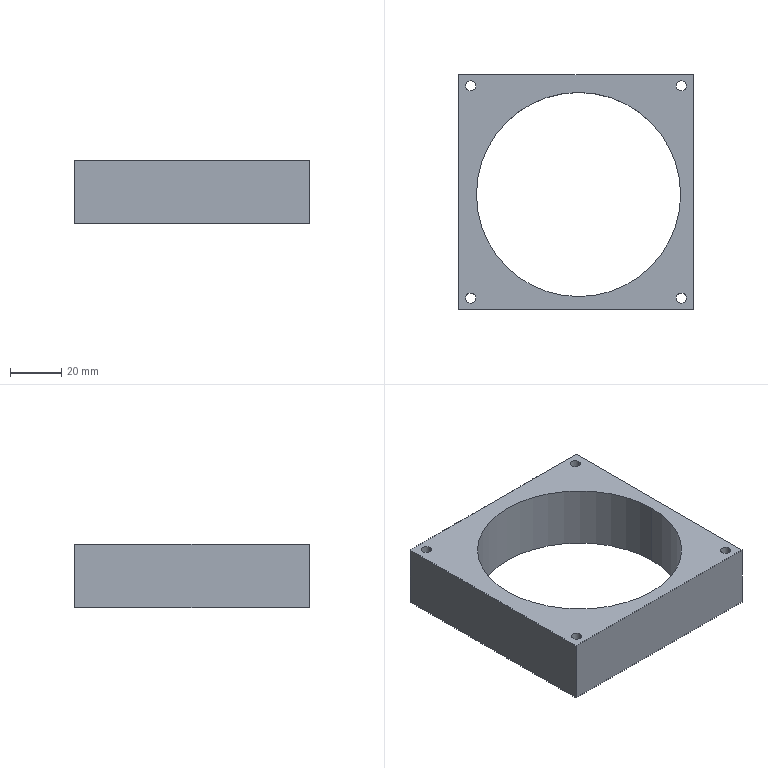Part | SolidWorks | features ICE 2, Extrusion 1 | 1 solid | 16 faces | box 92 x 92 x 25 mm | volume 84680 mm3 | cylinder 10 | plane 6 | commonest cylinder face diameters 4 x8 80 x2
STEP:
#1=CARTESIAN_POINT('',(-6.75,4.4,0.));
#2=VERTEX_POINT('',#1);
#3=CARTESIAN_POINT('',(-2.75,4.4,0.));
#4=VERTEX_POINT('',#3);
#5=CARTESIAN_POINT('',(-4.75,4.4,0.));
#6=DIRECTION('',(0.,0.,1.));
#7=DIRECTION('',(1.,0.,0.));
#8=AXIS2_PLACEMENT_3D('',#5,#6,#7);
#9=CIRCLE('',#8,2.);
#10=EDGE_CURVE('',#2,#4,#9,.T.);
#11=ORIENTED_EDGE('',*,*,#10,.F.);
#12=CARTESIAN_POINT('',(-6.75,4.4,25.));
#13=VERTEX_POINT('',#12);
#14=CARTESIAN_POINT('',(-6.75,4.4,-5.));
#15=DIRECTION('',(0.,0.,1.));
#16=VECTOR('',#15,1000.);
#17=LINE('',#14,#16);
#18=EDGE_CURVE('',#2,#13,#17,.T.);
#19=ORIENTED_EDGE('',*,*,#18,.T.);
#20=CARTESIAN_POINT('',(-2.75,4.4,25.));
#21=VERTEX_POINT('',#20);
#22=CARTESIAN_POINT('',(-4.75,4.4,25.));
#23=DIRECTION('',(0.,0.,1.));
#24=DIRECTION('',(-1.,0.,0.));
#25=AXIS2_PLACEMENT_3D('',#22,#23,#24);
#26=CIRCLE('',#25,2.);
#27=EDGE_CURVE('',#13,#21,#26,.T.);
#28=ORIENTED_EDGE('',*,*,#27,.T.);
#29=CARTESIAN_POINT('',(-2.75,4.4,-5.));
#30=DIRECTION('',(0.,0.,1.));
#31=VECTOR('',#30,1000.);
#32=LINE('',#29,#31);
#33=EDGE_CURVE('',#4,#21,#32,.T.);
#34=ORIENTED_EDGE('',*,*,#33,.F.);
#35=EDGE_LOOP('',(#11,#19,#28,#34));
#36=FACE_OUTER_BOUND('',#35,.T.);
#37=CARTESIAN_POINT('',(-4.75,4.4,-5.));
#38=DIRECTION('',(0.,0.,1.));
#39=DIRECTION('',(1.,0.,0.));
#40=AXIS2_PLACEMENT_3D('',#37,#38,#39);
#41=CYLINDRICAL_SURFACE('',#40,2.);
#42=ADVANCED_FACE('',(#36),#41,.F.);
#43=CARTESIAN_POINT('',(-89.25,4.4,0.));
#44=VERTEX_POINT('',#43);
#45=CARTESIAN_POINT('',(-85.25,4.4,0.));
#46=VERTEX_POINT('',#45);
#47=CARTESIAN_POINT('',(-87.25,4.4,0.));
#48=DIRECTION('',(0.,0.,1.));
#49=DIRECTION('',(1.,0.,0.));
#50=AXIS2_PLACEMENT_3D('',#47,#48,#49);
#51=CIRCLE('',#50,2.);
#52=EDGE_CURVE('',#44,#46,#51,.T.);
#53=ORIENTED_EDGE('',*,*,#52,.F.);
#54=CARTESIAN_POINT('',(-89.25,4.4,25.));
#55=VERTEX_POINT('',#54);
#56=CARTESIAN_POINT('',(-89.25,4.4,-5.));
#57=DIRECTION('',(0.,0.,1.));
#58=VECTOR('',#57,1000.);
#59=LINE('',#56,#58);
#60=EDGE_CURVE('',#44,#55,#59,.T.);
#61=ORIENTED_EDGE('',*,*,#60,.T.);
#62=CARTESIAN_POINT('',(-85.25,4.4,25.));
#63=VERTEX_POINT('',#62);
#64=CARTESIAN_POINT('',(-87.25,4.4,25.));
#65=DIRECTION('',(0.,0.,1.));
#66=DIRECTION('',(-1.,0.,0.));
#67=AXIS2_PLACEMENT_3D('',#64,#65,#66);
#68=CIRCLE('',#67,2.);
#69=EDGE_CURVE('',#55,#63,#68,.T.);
#70=ORIENTED_EDGE('',*,*,#69,.T.);
#71=CARTESIAN_POINT('',(-85.25,4.4,-5.));
#72=DIRECTION('',(0.,0.,1.));
#73=VECTOR('',#72,1000.);
#74=LINE('',#71,#73);
#75=EDGE_CURVE('',#46,#63,#74,.T.);
#76=ORIENTED_EDGE('',*,*,#75,.F.);
#77=EDGE_LOOP('',(#53,#61,#70,#76));
#78=FACE_OUTER_BOUND('',#77,.T.);
#79=CARTESIAN_POINT('',(-87.25,4.4,-5.));
#80=DIRECTION('',(0.,0.,1.));
#81=DIRECTION('',(1.,0.,0.));
#82=AXIS2_PLACEMENT_3D('',#79,#80,#81);
#83=CYLINDRICAL_SURFACE('',#82,2.);
#84=ADVANCED_FACE('',(#78),#83,.F.);
#85=CARTESIAN_POINT('',(-89.25,87.6,0.));
#86=VERTEX_POINT('',#85);
#87=CARTESIAN_POINT('',(-85.25,87.6,0.));
#88=VERTEX_POINT('',#87);
#89=CARTESIAN_POINT('',(-87.25,87.6,0.));
#90=DIRECTION('',(0.,0.,1.));
#91=DIRECTION('',(1.,0.,0.));
#92=AXIS2_PLACEMENT_3D('',#89,#90,#91);
#93=CIRCLE('',#92,2.);
#94=EDGE_CURVE('',#86,#88,#93,.T.);
#95=ORIENTED_EDGE('',*,*,#94,.F.);
#96=CARTESIAN_POINT('',(-89.25,87.6,25.));
#97=VERTEX_POINT('',#96);
#98=CARTESIAN_POINT('',(-89.25,87.6,-5.));
#99=DIRECTION('',(0.,0.,1.));
#100=VECTOR('',#99,1000.);
#101=LINE('',#98,#100);
#102=EDGE_CURVE('',#86,#97,#101,.T.);
#103=ORIENTED_EDGE('',*,*,#102,.T.);
#104=CARTESIAN_POINT('',(-85.25,87.6,25.));
#105=VERTEX_POINT('',#104);
#106=CARTESIAN_POINT('',(-87.25,87.6,25.));
#107=DIRECTION('',(0.,0.,1.));
#108=DIRECTION('',(1.,0.,0.));
#109=AXIS2_PLACEMENT_3D('',#106,#107,#108);
#110=CIRCLE('',#109,2.);
#111=EDGE_CURVE('',#97,#105,#110,.T.);
#112=ORIENTED_EDGE('',*,*,#111,.T.);
#113=CARTESIAN_POINT('',(-85.25,87.6,-5.));
#114=DIRECTION('',(0.,0.,1.));
#115=VECTOR('',#114,1000.);
#116=LINE('',#113,#115);
#117=EDGE_CURVE('',#88,#105,#116,.T.);
#118=ORIENTED_EDGE('',*,*,#117,.F.);
#119=EDGE_LOOP('',(#95,#103,#112,#118));
#120=FACE_OUTER_BOUND('',#119,.T.);
#121=CARTESIAN_POINT('',(-87.25,87.6,-5.));
#122=DIRECTION('',(0.,0.,1.));
#123=DIRECTION('',(1.,0.,0.));
#124=AXIS2_PLACEMENT_3D('',#121,#122,#123);
#125=CYLINDRICAL_SURFACE('',#124,2.);
#126=ADVANCED_FACE('',(#120),#125,.F.);
#127=CARTESIAN_POINT('',(-6.75,87.6,0.));
#128=VERTEX_POINT('',#127);
#129=CARTESIAN_POINT('',(-2.75,87.6,0.));
#130=VERTEX_POINT('',#129);
#131=CARTESIAN_POINT('',(-4.75,87.6,0.));
#132=DIRECTION('',(0.,0.,1.));
#133=DIRECTION('',(1.,0.,0.));
#134=AXIS2_PLACEMENT_3D('',#131,#132,#133);
#135=CIRCLE('',#134,2.);
#136=EDGE_CURVE('',#128,#130,#135,.T.);
#137=ORIENTED_EDGE('',*,*,#136,.F.);
#138=CARTESIAN_POINT('',(-6.75,87.6,25.));
#139=VERTEX_POINT('',#138);
#140=CARTESIAN_POINT('',(-6.75,87.6,-5.));
#141=DIRECTION('',(0.,0.,1.));
#142=VECTOR('',#141,1000.);
#143=LINE('',#140,#142);
#144=EDGE_CURVE('',#128,#139,#143,.T.);
#145=ORIENTED_EDGE('',*,*,#144,.T.);
#146=CARTESIAN_POINT('',(-2.75,87.6,25.));
#147=VERTEX_POINT('',#146);
#148=CARTESIAN_POINT('',(-4.75,87.6,25.));
#149=DIRECTION('',(0.,0.,1.));
#150=DIRECTION('',(1.,0.,0.));
#151=AXIS2_PLACEMENT_3D('',#148,#149,#150);
#152=CIRCLE('',#151,2.);
#153=EDGE_CURVE('',#139,#147,#152,.T.);
#154=ORIENTED_EDGE('',*,*,#153,.T.);
#155=CARTESIAN_POINT('',(-2.75,87.6,-5.));
#156=DIRECTION('',(0.,0.,1.));
#157=VECTOR('',#156,1000.);
#158=LINE('',#155,#157);
#159=EDGE_CURVE('',#130,#147,#158,.T.);
#160=ORIENTED_EDGE('',*,*,#159,.F.);
#161=EDGE_LOOP('',(#137,#145,#154,#160));
#162=FACE_OUTER_BOUND('',#161,.T.);
#163=CARTESIAN_POINT('',(-4.75,87.6,-5.));
#164=DIRECTION('',(0.,0.,1.));
#165=DIRECTION('',(1.,0.,0.));
#166=AXIS2_PLACEMENT_3D('',#163,#164,#165);
#167=CYLINDRICAL_SURFACE('',#166,2.);
#168=ADVANCED_FACE('',(#162),#167,.F.);
#169=CARTESIAN_POINT('',(-85.,45.,0.));
#170=VERTEX_POINT('',#169);
#171=CARTESIAN_POINT('',(-5.,45.,0.));
#172=VERTEX_POINT('',#171);
#173=CARTESIAN_POINT('',(-45.,45.,0.));
#174=DIRECTION('',(0.,0.,1.));
#175=DIRECTION('',(1.,0.,0.));
#176=AXIS2_PLACEMENT_3D('',#173,#174,#175);
#177=CIRCLE('',#176,40.);
#178=EDGE_CURVE('',#170,#172,#177,.T.);
#179=ORIENTED_EDGE('',*,*,#178,.F.);
#180=CARTESIAN_POINT('',(-85.,45.,25.));
#181=VERTEX_POINT('',#180);
#182=CARTESIAN_POINT('',(-85.,45.,0.));
#183=DIRECTION('',(0.,0.,1.));
#184=VECTOR('',#183,1000.);
#185=LINE('',#182,#184);
#186=EDGE_CURVE('',#170,#181,#185,.T.);
#187=ORIENTED_EDGE('',*,*,#186,.T.);
#188=CARTESIAN_POINT('',(-5.,45.,25.));
#189=VERTEX_POINT('',#188);
#190=CARTESIAN_POINT('',(-45.,45.,25.));
#191=DIRECTION('',(0.,0.,1.));
#192=DIRECTION('',(1.,0.,0.));
#193=AXIS2_PLACEMENT_3D('',#190,#191,#192);
#194=CIRCLE('',#193,40.);
#195=EDGE_CURVE('',#181,#189,#194,.T.);
#196=ORIENTED_EDGE('',*,*,#195,.T.);
#197=CARTESIAN_POINT('',(-5.,45.,0.));
#198=DIRECTION('',(0.,0.,1.));
#199=VECTOR('',#198,1000.);
#200=LINE('',#197,#199);
#201=EDGE_CURVE('',#172,#189,#200,.T.);
#202=ORIENTED_EDGE('',*,*,#201,.F.);
#203=EDGE_LOOP('',(#179,#187,#196,#202));
#204=FACE_OUTER_BOUND('',#203,.T.);
#205=CARTESIAN_POINT('',(-45.,45.,0.));
#206=DIRECTION('',(0.,0.,1.));
#207=DIRECTION('',(1.,0.,0.));
#208=AXIS2_PLACEMENT_3D('',#205,#206,#207);
#209=CYLINDRICAL_SURFACE('',#208,40.);
#210=ADVANCED_FACE('',(#204),#209,.F.);
#211=CARTESIAN_POINT('',(0.,0.,0.));
#212=VERTEX_POINT('',#211);
#213=CARTESIAN_POINT('',(0.,92.,0.));
#214=VERTEX_POINT('',#213);
#215=CARTESIAN_POINT('',(0.,0.,0.));
#216=DIRECTION('',(0.,1.,0.));
#217=VECTOR('',#216,1000.);
#218=LINE('',#215,#217);
#219=EDGE_CURVE('',#212,#214,#218,.T.);
#220=ORIENTED_EDGE('',*,*,#219,.T.);
#221=CARTESIAN_POINT('',(0.,92.,25.));
#222=VERTEX_POINT('',#221);
#223=CARTESIAN_POINT('',(0.,92.,25.));
#224=DIRECTION('',(0.,0.,-1.));
#225=VECTOR('',#224,1000.);
#226=LINE('',#223,#225);
#227=EDGE_CURVE('',#222,#214,#226,.T.);
#228=ORIENTED_EDGE('',*,*,#227,.F.);
#229=CARTESIAN_POINT('',(0.,0.,25.));
#230=VERTEX_POINT('',#229);
#231=CARTESIAN_POINT('',(0.,0.,25.));
#232=DIRECTION('',(0.,1.,0.));
#233=VECTOR('',#232,1000.);
#234=LINE('',#231,#233);
#235=EDGE_CURVE('',#230,#222,#234,.T.);
#236=ORIENTED_EDGE('',*,*,#235,.F.);
#237=CARTESIAN_POINT('',(0.,0.,25.));
#238=DIRECTION('',(0.,0.,-1.));
#239=VECTOR('',#238,1000.);
#240=LINE('',#237,#239);
#241=EDGE_CURVE('',#230,#212,#240,.T.);
#242=ORIENTED_EDGE('',*,*,#241,.T.);
#243=EDGE_LOOP('',(#220,#228,#236,#242));
#244=FACE_OUTER_BOUND('',#243,.T.);
#245=CARTESIAN_POINT('',(0.,0.,25.));
#246=DIRECTION('',(-1.,0.,0.));
#247=DIRECTION('',(0.,-1.,0.));
#248=AXIS2_PLACEMENT_3D('',#245,#246,#247);
#249=PLANE('',#248);
#250=ADVANCED_FACE('',(#244),#249,.F.);
#251=CARTESIAN_POINT('',(-92.,92.,0.));
#252=VERTEX_POINT('',#251);
#253=CARTESIAN_POINT('',(0.,92.,0.));
#254=DIRECTION('',(-1.,0.,0.));
#255=VECTOR('',#254,1000.);
#256=LINE('',#253,#255);
#257=EDGE_CURVE('',#214,#252,#256,.T.);
#258=ORIENTED_EDGE('',*,*,#257,.T.);
#259=CARTESIAN_POINT('',(-92.,92.,25.));
#260=VERTEX_POINT('',#259);
#261=CARTESIAN_POINT('',(-92.,92.,25.));
#262=DIRECTION('',(0.,0.,-1.));
#263=VECTOR('',#262,1000.);
#264=LINE('',#261,#263);
#265=EDGE_CURVE('',#260,#252,#264,.T.);
#266=ORIENTED_EDGE('',*,*,#265,.F.);
#267=CARTESIAN_POINT('',(0.,92.,25.));
#268=DIRECTION('',(-1.,0.,0.));
#269=VECTOR('',#268,1000.);
#270=LINE('',#267,#269);
#271=EDGE_CURVE('',#222,#260,#270,.T.);
#272=ORIENTED_EDGE('',*,*,#271,.F.);
#273=ORIENTED_EDGE('',*,*,#227,.T.);
#274=EDGE_LOOP('',(#258,#266,#272,#273));
#275=FACE_OUTER_BOUND('',#274,.T.);
#276=CARTESIAN_POINT('',(0.,92.,25.));
#277=DIRECTION('',(0.,-1.,0.));
#278=DIRECTION('',(0.,0.,-1.));
#279=AXIS2_PLACEMENT_3D('',#276,#277,#278);
#280=PLANE('',#279);
#281=ADVANCED_FACE('',(#275),#280,.F.);
#282=CARTESIAN_POINT('',(-92.,0.,0.));
#283=VERTEX_POINT('',#282);
#284=CARTESIAN_POINT('',(-92.,0.,0.));
#285=DIRECTION('',(0.,-1.,0.));
#286=VECTOR('',#285,1000.);
#287=LINE('',#284,#286);
#288=EDGE_CURVE('',#252,#283,#287,.T.);
#289=ORIENTED_EDGE('',*,*,#288,.T.);
#290=CARTESIAN_POINT('',(-92.,0.,25.));
#291=VERTEX_POINT('',#290);
#292=CARTESIAN_POINT('',(-92.,0.,25.));
#293=DIRECTION('',(0.,0.,-1.));
#294=VECTOR('',#293,1000.);
#295=LINE('',#292,#294);
#296=EDGE_CURVE('',#291,#283,#295,.T.);
#297=ORIENTED_EDGE('',*,*,#296,.F.);
#298=CARTESIAN_POINT('',(-92.,0.,25.));
#299=DIRECTION('',(0.,-1.,0.));
#300=VECTOR('',#299,1000.);
#301=LINE('',#298,#300);
#302=EDGE_CURVE('',#260,#291,#301,.T.);
#303=ORIENTED_EDGE('',*,*,#302,.F.);
#304=ORIENTED_EDGE('',*,*,#265,.T.);
#305=EDGE_LOOP('',(#289,#297,#303,#304));
#306=FACE_OUTER_BOUND('',#305,.T.);
#307=CARTESIAN_POINT('',(-92.,0.,25.));
#308=DIRECTION('',(1.,0.,0.));
#309=DIRECTION('',(0.,1.,0.));
#310=AXIS2_PLACEMENT_3D('',#307,#308,#309);
#311=PLANE('',#310);
#312=ADVANCED_FACE('',(#306),#311,.F.);
#313=CARTESIAN_POINT('',(0.,0.,0.));
#314=DIRECTION('',(1.,0.,0.));
#315=VECTOR('',#314,1000.);
#316=LINE('',#313,#315);
#317=EDGE_CURVE('',#283,#212,#316,.T.);
#318=ORIENTED_EDGE('',*,*,#317,.T.);
#319=ORIENTED_EDGE('',*,*,#241,.F.);
#320=CARTESIAN_POINT('',(0.,0.,25.));
#321=DIRECTION('',(1.,0.,0.));
#322=VECTOR('',#321,1000.);
#323=LINE('',#320,#322);
#324=EDGE_CURVE('',#291,#230,#323,.T.);
#325=ORIENTED_EDGE('',*,*,#324,.F.);
#326=ORIENTED_EDGE('',*,*,#296,.T.);
#327=EDGE_LOOP('',(#318,#319,#325,#326));
#328=FACE_OUTER_BOUND('',#327,.T.);
#329=CARTESIAN_POINT('',(0.,0.,25.));
#330=DIRECTION('',(0.,1.,0.));
#331=DIRECTION('',(-1.,0.,0.));
#332=AXIS2_PLACEMENT_3D('',#329,#330,#331);
#333=PLANE('',#332);
#334=ADVANCED_FACE('',(#328),#333,.F.);
#335=CARTESIAN_POINT('',(-4.75,4.4,25.));
#336=DIRECTION('',(0.,0.,1.));
#337=DIRECTION('',(-1.,0.,0.));
#338=AXIS2_PLACEMENT_3D('',#335,#336,#337);
#339=CIRCLE('',#338,2.);
#340=EDGE_CURVE('',#21,#13,#339,.T.);
#341=ORIENTED_EDGE('',*,*,#340,.F.);
#342=ORIENTED_EDGE('',*,*,#27,.F.);
#343=EDGE_LOOP('',(#341,#342));
#344=FACE_BOUND('',#343,.T.);
#345=CARTESIAN_POINT('',(-87.25,4.4,25.));
#346=DIRECTION('',(0.,0.,1.));
#347=DIRECTION('',(-1.,0.,0.));
#348=AXIS2_PLACEMENT_3D('',#345,#346,#347);
#349=CIRCLE('',#348,2.);
#350=EDGE_CURVE('',#63,#55,#349,.T.);
#351=ORIENTED_EDGE('',*,*,#350,.F.);
#352=ORIENTED_EDGE('',*,*,#69,.F.);
#353=EDGE_LOOP('',(#351,#352));
#354=FACE_BOUND('',#353,.T.);
#355=CARTESIAN_POINT('',(-87.25,87.6,25.));
#356=DIRECTION('',(0.,0.,1.));
#357=DIRECTION('',(1.,0.,0.));
#358=AXIS2_PLACEMENT_3D('',#355,#356,#357);
#359=CIRCLE('',#358,2.);
#360=EDGE_CURVE('',#105,#97,#359,.T.);
#361=ORIENTED_EDGE('',*,*,#360,.F.);
#362=ORIENTED_EDGE('',*,*,#111,.F.);
#363=EDGE_LOOP('',(#361,#362));
#364=FACE_BOUND('',#363,.T.);
#365=CARTESIAN_POINT('',(-4.75,87.6,25.));
#366=DIRECTION('',(0.,0.,1.));
#367=DIRECTION('',(1.,0.,0.));
#368=AXIS2_PLACEMENT_3D('',#365,#366,#367);
#369=CIRCLE('',#368,2.);
#370=EDGE_CURVE('',#147,#139,#369,.T.);
#371=ORIENTED_EDGE('',*,*,#370,.F.);
#372=ORIENTED_EDGE('',*,*,#153,.F.);
#373=EDGE_LOOP('',(#371,#372));
#374=FACE_BOUND('',#373,.T.);
#375=CARTESIAN_POINT('',(-45.,45.,25.));
#376=DIRECTION('',(0.,0.,1.));
#377=DIRECTION('',(1.,0.,0.));
#378=AXIS2_PLACEMENT_3D('',#375,#376,#377);
#379=CIRCLE('',#378,40.);
#380=EDGE_CURVE('',#189,#181,#379,.T.);
#381=ORIENTED_EDGE('',*,*,#380,.F.);
#382=ORIENTED_EDGE('',*,*,#195,.F.);
#383=EDGE_LOOP('',(#381,#382));
#384=FACE_BOUND('',#383,.T.);
#385=ORIENTED_EDGE('',*,*,#235,.T.);
#386=ORIENTED_EDGE('',*,*,#271,.T.);
#387=ORIENTED_EDGE('',*,*,#302,.T.);
#388=ORIENTED_EDGE('',*,*,#324,.T.);
#389=EDGE_LOOP('',(#385,#386,#387,#388));
#390=FACE_OUTER_BOUND('',#389,.T.);
#391=CARTESIAN_POINT('',(0.,0.,25.));
#392=DIRECTION('',(0.,0.,1.));
#393=DIRECTION('',(1.,0.,0.));
#394=AXIS2_PLACEMENT_3D('',#391,#392,#393);
#395=PLANE('',#394);
#396=ADVANCED_FACE('',(#344,#354,#364,#374,#384,#390),#395,.T.);
#397=CARTESIAN_POINT('',(-4.75,4.4,0.));
#398=DIRECTION('',(0.,0.,1.));
#399=DIRECTION('',(1.,0.,0.));
#400=AXIS2_PLACEMENT_3D('',#397,#398,#399);
#401=CIRCLE('',#400,2.);
#402=EDGE_CURVE('',#4,#2,#401,.T.);
#403=ORIENTED_EDGE('',*,*,#402,.T.);
#404=ORIENTED_EDGE('',*,*,#10,.T.);
#405=EDGE_LOOP('',(#403,#404));
#406=FACE_BOUND('',#405,.T.);
#407=CARTESIAN_POINT('',(-87.25,4.4,0.));
#408=DIRECTION('',(0.,0.,1.));
#409=DIRECTION('',(1.,0.,0.));
#410=AXIS2_PLACEMENT_3D('',#407,#408,#409);
#411=CIRCLE('',#410,2.);
#412=EDGE_CURVE('',#46,#44,#411,.T.);
#413=ORIENTED_EDGE('',*,*,#412,.T.);
#414=ORIENTED_EDGE('',*,*,#52,.T.);
#415=EDGE_LOOP('',(#413,#414));
#416=FACE_BOUND('',#415,.T.);
#417=CARTESIAN_POINT('',(-87.25,87.6,0.));
#418=DIRECTION('',(0.,0.,1.));
#419=DIRECTION('',(1.,0.,0.));
#420=AXIS2_PLACEMENT_3D('',#417,#418,#419);
#421=CIRCLE('',#420,2.);
#422=EDGE_CURVE('',#88,#86,#421,.T.);
#423=ORIENTED_EDGE('',*,*,#422,.T.);
#424=ORIENTED_EDGE('',*,*,#94,.T.);
#425=EDGE_LOOP('',(#423,#424));
#426=FACE_BOUND('',#425,.T.);
#427=CARTESIAN_POINT('',(-4.75,87.6,0.));
#428=DIRECTION('',(0.,0.,1.));
#429=DIRECTION('',(1.,0.,0.));
#430=AXIS2_PLACEMENT_3D('',#427,#428,#429);
#431=CIRCLE('',#430,2.);
#432=EDGE_CURVE('',#130,#128,#431,.T.);
#433=ORIENTED_EDGE('',*,*,#432,.T.);
#434=ORIENTED_EDGE('',*,*,#136,.T.);
#435=EDGE_LOOP('',(#433,#434));
#436=FACE_BOUND('',#435,.T.);
#437=CARTESIAN_POINT('',(-45.,45.,0.));
#438=DIRECTION('',(0.,0.,1.));
#439=DIRECTION('',(1.,0.,0.));
#440=AXIS2_PLACEMENT_3D('',#437,#438,#439);
#441=CIRCLE('',#440,40.);
#442=EDGE_CURVE('',#172,#170,#441,.T.);
#443=ORIENTED_EDGE('',*,*,#442,.T.);
#444=ORIENTED_EDGE('',*,*,#178,.T.);
#445=EDGE_LOOP('',(#443,#444));
#446=FACE_BOUND('',#445,.T.);
#447=ORIENTED_EDGE('',*,*,#219,.F.);
#448=ORIENTED_EDGE('',*,*,#317,.F.);
#449=ORIENTED_EDGE('',*,*,#288,.F.);
#450=ORIENTED_EDGE('',*,*,#257,.F.);
#451=EDGE_LOOP('',(#447,#448,#449,#450));
#452=FACE_OUTER_BOUND('',#451,.T.);
#453=CARTESIAN_POINT('',(0.,0.,0.));
#454=DIRECTION('',(0.,0.,1.));
#455=DIRECTION('',(1.,0.,0.));
#456=AXIS2_PLACEMENT_3D('',#453,#454,#455);
#457=PLANE('',#456);
#458=ADVANCED_FACE('',(#406,#416,#426,#436,#446,#452),#457,.F.);
#459=ORIENTED_EDGE('',*,*,#186,.F.);
#460=ORIENTED_EDGE('',*,*,#442,.F.);
#461=ORIENTED_EDGE('',*,*,#201,.T.);
#462=ORIENTED_EDGE('',*,*,#380,.T.);
#463=EDGE_LOOP('',(#459,#460,#461,#462));
#464=FACE_OUTER_BOUND('',#463,.T.);
#465=CARTESIAN_POINT('',(-45.,45.,0.));
#466=DIRECTION('',(0.,0.,1.));
#467=DIRECTION('',(1.,0.,0.));
#468=AXIS2_PLACEMENT_3D('',#465,#466,#467);
#469=CYLINDRICAL_SURFACE('',#468,40.);
#470=ADVANCED_FACE('',(#464),#469,.F.);
#471=ORIENTED_EDGE('',*,*,#144,.F.);
#472=ORIENTED_EDGE('',*,*,#432,.F.);
#473=ORIENTED_EDGE('',*,*,#159,.T.);
#474=ORIENTED_EDGE('',*,*,#370,.T.);
#475=EDGE_LOOP('',(#471,#472,#473,#474));
#476=FACE_OUTER_BOUND('',#475,.T.);
#477=CARTESIAN_POINT('',(-4.75,87.6,-5.));
#478=DIRECTION('',(0.,0.,1.));
#479=DIRECTION('',(1.,0.,0.));
#480=AXIS2_PLACEMENT_3D('',#477,#478,#479);
#481=CYLINDRICAL_SURFACE('',#480,2.);
#482=ADVANCED_FACE('',(#476),#481,.F.);
#483=ORIENTED_EDGE('',*,*,#102,.F.);
#484=ORIENTED_EDGE('',*,*,#422,.F.);
#485=ORIENTED_EDGE('',*,*,#117,.T.);
#486=ORIENTED_EDGE('',*,*,#360,.T.);
#487=EDGE_LOOP('',(#483,#484,#485,#486));
#488=FACE_OUTER_BOUND('',#487,.T.);
#489=CARTESIAN_POINT('',(-87.25,87.6,-5.));
#490=DIRECTION('',(0.,0.,1.));
#491=DIRECTION('',(1.,0.,0.));
#492=AXIS2_PLACEMENT_3D('',#489,#490,#491);
#493=CYLINDRICAL_SURFACE('',#492,2.);
#494=ADVANCED_FACE('',(#488),#493,.F.);
#495=ORIENTED_EDGE('',*,*,#60,.F.);
#496=ORIENTED_EDGE('',*,*,#412,.F.);
#497=ORIENTED_EDGE('',*,*,#75,.T.);
#498=ORIENTED_EDGE('',*,*,#350,.T.);
#499=EDGE_LOOP('',(#495,#496,#497,#498));
#500=FACE_OUTER_BOUND('',#499,.T.);
#501=CARTESIAN_POINT('',(-87.25,4.4,-5.));
#502=DIRECTION('',(0.,0.,1.));
#503=DIRECTION('',(1.,0.,0.));
#504=AXIS2_PLACEMENT_3D('',#501,#502,#503);
#505=CYLINDRICAL_SURFACE('',#504,2.);
#506=ADVANCED_FACE('',(#500),#505,.F.);
#507=ORIENTED_EDGE('',*,*,#18,.F.);
#508=ORIENTED_EDGE('',*,*,#402,.F.);
#509=ORIENTED_EDGE('',*,*,#33,.T.);
#510=ORIENTED_EDGE('',*,*,#340,.T.);
#511=EDGE_LOOP('',(#507,#508,#509,#510));
#512=FACE_OUTER_BOUND('',#511,.T.);
#513=CARTESIAN_POINT('',(-4.75,4.4,-5.));
#514=DIRECTION('',(0.,0.,1.));
#515=DIRECTION('',(1.,0.,0.));
#516=AXIS2_PLACEMENT_3D('',#513,#514,#515);
#517=CYLINDRICAL_SURFACE('',#516,2.);
#518=ADVANCED_FACE('',(#512),#517,.F.);
#519=CLOSED_SHELL('',(#42,#84,#126,#168,#210,#250,#281,#312,#334,#396,#458,#470,#482,#494,#506,#518));
#520=MANIFOLD_SOLID_BREP('',#519);
#521=CARTESIAN_POINT('',(0.,0.,0.));
#522=DIRECTION('',(0.,0.,1.));
#523=DIRECTION('',(1.,0.,0.));
#524=AXIS2_PLACEMENT_3D('',#521,#522,#523);
#525=(LENGTH_UNIT()NAMED_UNIT(*)SI_UNIT(.MILLI.,.METRE.));
#526=UNCERTAINTY_MEASURE_WITH_UNIT(LENGTH_MEASURE(0.00001),#525,'','');
#527=(NAMED_UNIT(*)PLANE_ANGLE_UNIT()SI_UNIT($,.RADIAN.));
#528=(NAMED_UNIT(*)SI_UNIT($,.STERADIAN.)SOLID_ANGLE_UNIT());
#529=(GEOMETRIC_REPRESENTATION_CONTEXT(3)GLOBAL_UNCERTAINTY_ASSIGNED_CONTEXT((#526))GLOBAL_UNIT_ASSIGNED_CONTEXT((#525,#527,#528))REPRESENTATION_CONTEXT('',''));
#530=ADVANCED_BREP_SHAPE_REPRESENTATION('',(#520,#524),#529);